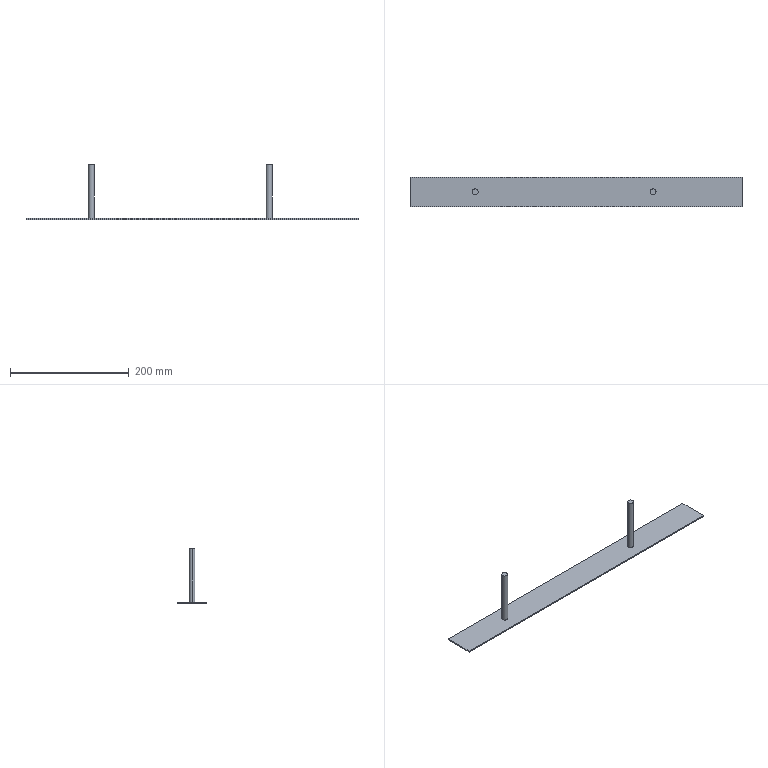Part | STEP file | 1 solid | 12 faces | box 560 x 50 x 93 mm | volume 70294 mm3 | plane 8 | cylinder 4 | commonest cylinder face diameters 10 x4
STEP:
#1=CARTESIAN_POINT('',(0.,0.,0.));
#2=DIRECTION('',(0.,0.,1.));
#3=DIRECTION('',(1.,0.,0.));
#4=AXIS2_PLACEMENT_3D('',#1,#2,#3);
#5=CARTESIAN_POINT('',(125.,0.,2.));
#6=VERTEX_POINT('',#5);
#7=CARTESIAN_POINT('',(135.,0.,2.));
#8=VERTEX_POINT('',#7);
#9=CARTESIAN_POINT('',(130.,0.,2.));
#10=DIRECTION('',(0.,0.,-1.));
#11=DIRECTION('',(1.,0.,0.));
#12=AXIS2_PLACEMENT_3D('',#9,#10,#11);
#13=CIRCLE('',#12,5.);
#14=CARTESIAN_POINT('',(130.,0.,93.));
#15=DIRECTION('',(0.,0.,1.));
#16=DIRECTION('',(1.,0.,0.));
#17=AXIS2_PLACEMENT_3D('',#14,#15,#16);
#18=CYLINDRICAL_SURFACE('',#17,5.);
#19=CARTESIAN_POINT('',(6.283,-91.));
#20=DIRECTION('',(-1.,0.));
#21=VECTOR('',#20,1.);
#22=LINE('',#19,#21);
#23=(GEOMETRIC_REPRESENTATION_CONTEXT(2)PARAMETRIC_REPRESENTATION_CONTEXT()REPRESENTATION_CONTEXT('',''));
#24=DEFINITIONAL_REPRESENTATION('',(#22),#23);
#25=PCURVE('',#18,#24);
#26=CARTESIAN_POINT('',(0.,0.,2.));
#27=DIRECTION('',(0.,0.,1.));
#28=DIRECTION('',(1.,0.,0.));
#29=AXIS2_PLACEMENT_3D('',#26,#27,#28);
#30=PLANE('',#29);
#31=CARTESIAN_POINT('',(135.,0.));
#32=CARTESIAN_POINT('',(135.,-8.66));
#33=CARTESIAN_POINT('',(127.5,-4.33));
#34=CARTESIAN_POINT('',(120.,0.));
#35=CARTESIAN_POINT('',(127.5,4.33));
#36=CARTESIAN_POINT('',(135.,8.66));
#37=CARTESIAN_POINT('',(135.,0.));
#38=(BOUNDED_CURVE()B_SPLINE_CURVE(2,(#31,#32,#33,#34,#35,#36,#37),.UNSPECIFIED.,.T.,.F.)B_SPLINE_CURVE_WITH_KNOTS((1,2,2,2,2,1),(-2.094,0.,2.094,4.189,6.283,8.378),.UNSPECIFIED.)CURVE()GEOMETRIC_REPRESENTATION_ITEM()RATIONAL_B_SPLINE_CURVE((1.,0.5,1.,0.5,1.,0.5,1.))REPRESENTATION_ITEM(''));
#39=(GEOMETRIC_REPRESENTATION_CONTEXT(2)PARAMETRIC_REPRESENTATION_CONTEXT()REPRESENTATION_CONTEXT('',''));
#40=DEFINITIONAL_REPRESENTATION('',(#38),#39);
#41=PCURVE('',#30,#40);
#42=SURFACE_CURVE('',#13,(#25,#41),.PCURVE_S1.);
#43=EDGE_CURVE('',#6,#8,#42,.T.);
#44=ORIENTED_EDGE('',*,*,#43,.F.);
#45=CARTESIAN_POINT('',(125.,0.,93.));
#46=VERTEX_POINT('',#45);
#47=CARTESIAN_POINT('',(125.,0.,93.));
#48=DIRECTION('',(0.,0.,1.));
#49=VECTOR('',#48,1.);
#50=LINE('',#47,#49);
#51=CARTESIAN_POINT('',(3.142,0.));
#52=DIRECTION('',(0.,1.));
#53=VECTOR('',#52,1.);
#54=LINE('',#51,#53);
#55=(GEOMETRIC_REPRESENTATION_CONTEXT(2)PARAMETRIC_REPRESENTATION_CONTEXT()REPRESENTATION_CONTEXT('',''));
#56=DEFINITIONAL_REPRESENTATION('',(#54),#55);
#57=PCURVE('',#18,#56);
#58=CARTESIAN_POINT('',(130.,0.,93.));
#59=DIRECTION('',(0.,0.,1.));
#60=DIRECTION('',(1.,0.,0.));
#61=AXIS2_PLACEMENT_3D('',#58,#59,#60);
#62=CYLINDRICAL_SURFACE('',#61,5.);
#63=CARTESIAN_POINT('',(3.142,0.));
#64=DIRECTION('',(0.,1.));
#65=VECTOR('',#64,1.);
#66=LINE('',#63,#65);
#67=(GEOMETRIC_REPRESENTATION_CONTEXT(2)PARAMETRIC_REPRESENTATION_CONTEXT()REPRESENTATION_CONTEXT('',''));
#68=DEFINITIONAL_REPRESENTATION('',(#66),#67);
#69=PCURVE('',#62,#68);
#70=SURFACE_CURVE('',#50,(#57,#69),.PCURVE_S1.);
#71=EDGE_CURVE('',#6,#46,#70,.T.);
#72=ORIENTED_EDGE('',*,*,#71,.T.);
#73=CARTESIAN_POINT('',(135.,0.,93.));
#74=VERTEX_POINT('',#73);
#75=CARTESIAN_POINT('',(130.,0.,93.));
#76=DIRECTION('',(0.,0.,-1.));
#77=DIRECTION('',(1.,0.,0.));
#78=AXIS2_PLACEMENT_3D('',#75,#76,#77);
#79=CIRCLE('',#78,5.);
#80=CARTESIAN_POINT('',(6.283,0.));
#81=DIRECTION('',(-1.,0.));
#82=VECTOR('',#81,1.);
#83=LINE('',#80,#82);
#84=(GEOMETRIC_REPRESENTATION_CONTEXT(2)PARAMETRIC_REPRESENTATION_CONTEXT()REPRESENTATION_CONTEXT('',''));
#85=DEFINITIONAL_REPRESENTATION('',(#83),#84);
#86=PCURVE('',#18,#85);
#87=CARTESIAN_POINT('',(130.,0.,93.));
#88=DIRECTION('',(0.,0.,1.));
#89=DIRECTION('',(1.,0.,0.));
#90=AXIS2_PLACEMENT_3D('',#87,#88,#89);
#91=PLANE('',#90);
#92=CARTESIAN_POINT('',(5.,0.));
#93=CARTESIAN_POINT('',(5.,-8.66));
#94=CARTESIAN_POINT('',(-2.5,-4.33));
#95=CARTESIAN_POINT('',(-10.,0.));
#96=CARTESIAN_POINT('',(-2.5,4.33));
#97=CARTESIAN_POINT('',(5.,8.66));
#98=CARTESIAN_POINT('',(5.,0.));
#99=(BOUNDED_CURVE()B_SPLINE_CURVE(2,(#92,#93,#94,#95,#96,#97,#98),.UNSPECIFIED.,.T.,.F.)B_SPLINE_CURVE_WITH_KNOTS((1,2,2,2,2,1),(-2.094,0.,2.094,4.189,6.283,8.378),.UNSPECIFIED.)CURVE()GEOMETRIC_REPRESENTATION_ITEM()RATIONAL_B_SPLINE_CURVE((1.,0.5,1.,0.5,1.,0.5,1.))REPRESENTATION_ITEM(''));
#100=(GEOMETRIC_REPRESENTATION_CONTEXT(2)PARAMETRIC_REPRESENTATION_CONTEXT()REPRESENTATION_CONTEXT('',''));
#101=DEFINITIONAL_REPRESENTATION('',(#99),#100);
#102=PCURVE('',#91,#101);
#103=SURFACE_CURVE('',#79,(#86,#102),.PCURVE_S1.);
#104=EDGE_CURVE('',#46,#74,#103,.T.);
#105=ORIENTED_EDGE('',*,*,#104,.T.);
#106=CARTESIAN_POINT('',(135.,0.,93.));
#107=DIRECTION('',(0.,0.,1.));
#108=VECTOR('',#107,1.);
#109=LINE('',#106,#108);
#110=CARTESIAN_POINT('',(0.,0.));
#111=DIRECTION('',(0.,1.));
#112=VECTOR('',#111,1.);
#113=LINE('',#110,#112);
#114=(GEOMETRIC_REPRESENTATION_CONTEXT(2)PARAMETRIC_REPRESENTATION_CONTEXT()REPRESENTATION_CONTEXT('',''));
#115=DEFINITIONAL_REPRESENTATION('',(#113),#114);
#116=PCURVE('',#18,#115);
#117=CARTESIAN_POINT('',(6.283,0.));
#118=DIRECTION('',(0.,1.));
#119=VECTOR('',#118,1.);
#120=LINE('',#117,#119);
#121=(GEOMETRIC_REPRESENTATION_CONTEXT(2)PARAMETRIC_REPRESENTATION_CONTEXT()REPRESENTATION_CONTEXT('',''));
#122=DEFINITIONAL_REPRESENTATION('',(#120),#121);
#123=PCURVE('',#62,#122);
#124=SURFACE_CURVE('',#109,(#116,#123),.PCURVE_S1.);
#125=EDGE_CURVE('',#8,#74,#124,.T.);
#126=ORIENTED_EDGE('',*,*,#125,.F.);
#127=EDGE_LOOP('',(#44,#72,#105,#126));
#128=FACE_BOUND('',#127,.T.);
#129=ADVANCED_FACE('',(#128),#18,.T.);
#130=CARTESIAN_POINT('',(-175.,0.,2.));
#131=VERTEX_POINT('',#130);
#132=CARTESIAN_POINT('',(-165.,0.,2.));
#133=VERTEX_POINT('',#132);
#134=CARTESIAN_POINT('',(-170.,0.,2.));
#135=DIRECTION('',(0.,0.,-1.));
#136=DIRECTION('',(1.,0.,0.));
#137=AXIS2_PLACEMENT_3D('',#134,#135,#136);
#138=CIRCLE('',#137,5.);
#139=CARTESIAN_POINT('',(-170.,0.,93.));
#140=DIRECTION('',(0.,0.,1.));
#141=DIRECTION('',(1.,0.,0.));
#142=AXIS2_PLACEMENT_3D('',#139,#140,#141);
#143=CYLINDRICAL_SURFACE('',#142,5.);
#144=CARTESIAN_POINT('',(6.283,-91.));
#145=DIRECTION('',(-1.,0.));
#146=VECTOR('',#145,1.);
#147=LINE('',#144,#146);
#148=(GEOMETRIC_REPRESENTATION_CONTEXT(2)PARAMETRIC_REPRESENTATION_CONTEXT()REPRESENTATION_CONTEXT('',''));
#149=DEFINITIONAL_REPRESENTATION('',(#147),#148);
#150=PCURVE('',#143,#149);
#151=CARTESIAN_POINT('',(-165.,0.));
#152=CARTESIAN_POINT('',(-165.,-8.66));
#153=CARTESIAN_POINT('',(-172.5,-4.33));
#154=CARTESIAN_POINT('',(-180.,0.));
#155=CARTESIAN_POINT('',(-172.5,4.33));
#156=CARTESIAN_POINT('',(-165.,8.66));
#157=CARTESIAN_POINT('',(-165.,0.));
#158=(BOUNDED_CURVE()B_SPLINE_CURVE(2,(#151,#152,#153,#154,#155,#156,#157),.UNSPECIFIED.,.T.,.F.)B_SPLINE_CURVE_WITH_KNOTS((1,2,2,2,2,1),(-2.094,0.,2.094,4.189,6.283,8.378),.UNSPECIFIED.)CURVE()GEOMETRIC_REPRESENTATION_ITEM()RATIONAL_B_SPLINE_CURVE((1.,0.5,1.,0.5,1.,0.5,1.))REPRESENTATION_ITEM(''));
#159=(GEOMETRIC_REPRESENTATION_CONTEXT(2)PARAMETRIC_REPRESENTATION_CONTEXT()REPRESENTATION_CONTEXT('',''));
#160=DEFINITIONAL_REPRESENTATION('',(#158),#159);
#161=PCURVE('',#30,#160);
#162=SURFACE_CURVE('',#138,(#150,#161),.PCURVE_S1.);
#163=EDGE_CURVE('',#131,#133,#162,.T.);
#164=ORIENTED_EDGE('',*,*,#163,.F.);
#165=CARTESIAN_POINT('',(-175.,0.,93.));
#166=VERTEX_POINT('',#165);
#167=CARTESIAN_POINT('',(-175.,0.,93.));
#168=DIRECTION('',(0.,0.,1.));
#169=VECTOR('',#168,1.);
#170=LINE('',#167,#169);
#171=CARTESIAN_POINT('',(3.142,0.));
#172=DIRECTION('',(0.,1.));
#173=VECTOR('',#172,1.);
#174=LINE('',#171,#173);
#175=(GEOMETRIC_REPRESENTATION_CONTEXT(2)PARAMETRIC_REPRESENTATION_CONTEXT()REPRESENTATION_CONTEXT('',''));
#176=DEFINITIONAL_REPRESENTATION('',(#174),#175);
#177=PCURVE('',#143,#176);
#178=CARTESIAN_POINT('',(-170.,0.,93.));
#179=DIRECTION('',(0.,0.,1.));
#180=DIRECTION('',(1.,0.,0.));
#181=AXIS2_PLACEMENT_3D('',#178,#179,#180);
#182=CYLINDRICAL_SURFACE('',#181,5.);
#183=CARTESIAN_POINT('',(3.142,0.));
#184=DIRECTION('',(0.,1.));
#185=VECTOR('',#184,1.);
#186=LINE('',#183,#185);
#187=(GEOMETRIC_REPRESENTATION_CONTEXT(2)PARAMETRIC_REPRESENTATION_CONTEXT()REPRESENTATION_CONTEXT('',''));
#188=DEFINITIONAL_REPRESENTATION('',(#186),#187);
#189=PCURVE('',#182,#188);
#190=SURFACE_CURVE('',#170,(#177,#189),.PCURVE_S1.);
#191=EDGE_CURVE('',#131,#166,#190,.T.);
#192=ORIENTED_EDGE('',*,*,#191,.T.);
#193=CARTESIAN_POINT('',(-165.,0.,93.));
#194=VERTEX_POINT('',#193);
#195=CARTESIAN_POINT('',(-170.,0.,93.));
#196=DIRECTION('',(0.,0.,-1.));
#197=DIRECTION('',(1.,0.,0.));
#198=AXIS2_PLACEMENT_3D('',#195,#196,#197);
#199=CIRCLE('',#198,5.);
#200=CARTESIAN_POINT('',(6.283,0.));
#201=DIRECTION('',(-1.,0.));
#202=VECTOR('',#201,1.);
#203=LINE('',#200,#202);
#204=(GEOMETRIC_REPRESENTATION_CONTEXT(2)PARAMETRIC_REPRESENTATION_CONTEXT()REPRESENTATION_CONTEXT('',''));
#205=DEFINITIONAL_REPRESENTATION('',(#203),#204);
#206=PCURVE('',#143,#205);
#207=CARTESIAN_POINT('',(-170.,0.,93.));
#208=DIRECTION('',(0.,0.,1.));
#209=DIRECTION('',(1.,0.,0.));
#210=AXIS2_PLACEMENT_3D('',#207,#208,#209);
#211=PLANE('',#210);
#212=CARTESIAN_POINT('',(5.,0.));
#213=CARTESIAN_POINT('',(5.,-8.66));
#214=CARTESIAN_POINT('',(-2.5,-4.33));
#215=CARTESIAN_POINT('',(-10.,0.));
#216=CARTESIAN_POINT('',(-2.5,4.33));
#217=CARTESIAN_POINT('',(5.,8.66));
#218=CARTESIAN_POINT('',(5.,0.));
#219=(BOUNDED_CURVE()B_SPLINE_CURVE(2,(#212,#213,#214,#215,#216,#217,#218),.UNSPECIFIED.,.T.,.F.)B_SPLINE_CURVE_WITH_KNOTS((1,2,2,2,2,1),(-2.094,0.,2.094,4.189,6.283,8.378),.UNSPECIFIED.)CURVE()GEOMETRIC_REPRESENTATION_ITEM()RATIONAL_B_SPLINE_CURVE((1.,0.5,1.,0.5,1.,0.5,1.))REPRESENTATION_ITEM(''));
#220=(GEOMETRIC_REPRESENTATION_CONTEXT(2)PARAMETRIC_REPRESENTATION_CONTEXT()REPRESENTATION_CONTEXT('',''));
#221=DEFINITIONAL_REPRESENTATION('',(#219),#220);
#222=PCURVE('',#211,#221);
#223=SURFACE_CURVE('',#199,(#206,#222),.PCURVE_S1.);
#224=EDGE_CURVE('',#166,#194,#223,.T.);
#225=ORIENTED_EDGE('',*,*,#224,.T.);
#226=CARTESIAN_POINT('',(-165.,0.,93.));
#227=DIRECTION('',(0.,0.,1.));
#228=VECTOR('',#227,1.);
#229=LINE('',#226,#228);
#230=CARTESIAN_POINT('',(0.,0.));
#231=DIRECTION('',(0.,1.));
#232=VECTOR('',#231,1.);
#233=LINE('',#230,#232);
#234=(GEOMETRIC_REPRESENTATION_CONTEXT(2)PARAMETRIC_REPRESENTATION_CONTEXT()REPRESENTATION_CONTEXT('',''));
#235=DEFINITIONAL_REPRESENTATION('',(#233),#234);
#236=PCURVE('',#143,#235);
#237=CARTESIAN_POINT('',(6.283,0.));
#238=DIRECTION('',(0.,1.));
#239=VECTOR('',#238,1.);
#240=LINE('',#237,#239);
#241=(GEOMETRIC_REPRESENTATION_CONTEXT(2)PARAMETRIC_REPRESENTATION_CONTEXT()REPRESENTATION_CONTEXT('',''));
#242=DEFINITIONAL_REPRESENTATION('',(#240),#241);
#243=PCURVE('',#182,#242);
#244=SURFACE_CURVE('',#229,(#236,#243),.PCURVE_S1.);
#245=EDGE_CURVE('',#133,#194,#244,.T.);
#246=ORIENTED_EDGE('',*,*,#245,.F.);
#247=EDGE_LOOP('',(#164,#192,#225,#246));
#248=FACE_BOUND('',#247,.T.);
#249=ADVANCED_FACE('',(#248),#143,.T.);
#250=CARTESIAN_POINT('',(-280.,-25.,0.));
#251=VERTEX_POINT('',#250);
#252=CARTESIAN_POINT('',(280.,-25.,0.));
#253=VERTEX_POINT('',#252);
#254=CARTESIAN_POINT('',(0.,-25.,0.));
#255=DIRECTION('',(1.,0.,0.));
#256=VECTOR('',#255,1.);
#257=LINE('',#254,#256);
#258=CARTESIAN_POINT('',(0.,0.,0.));
#259=DIRECTION('',(0.,0.,1.));
#260=DIRECTION('',(1.,0.,0.));
#261=AXIS2_PLACEMENT_3D('',#258,#259,#260);
#262=PLANE('',#261);
#263=CARTESIAN_POINT('',(0.,-25.));
#264=DIRECTION('',(1.,0.));
#265=VECTOR('',#264,1.);
#266=LINE('',#263,#265);
#267=(GEOMETRIC_REPRESENTATION_CONTEXT(2)PARAMETRIC_REPRESENTATION_CONTEXT()REPRESENTATION_CONTEXT('',''));
#268=DEFINITIONAL_REPRESENTATION('',(#266),#267);
#269=PCURVE('',#262,#268);
#270=CARTESIAN_POINT('',(-280.,-25.,2.));
#271=DIRECTION('',(0.,1.,0.));
#272=DIRECTION('',(0.,0.,1.));
#273=AXIS2_PLACEMENT_3D('',#270,#271,#272);
#274=PLANE('',#273);
#275=CARTESIAN_POINT('',(-2.,280.));
#276=DIRECTION('',(0.,1.));
#277=VECTOR('',#276,1.);
#278=LINE('',#275,#277);
#279=(GEOMETRIC_REPRESENTATION_CONTEXT(2)PARAMETRIC_REPRESENTATION_CONTEXT()REPRESENTATION_CONTEXT('',''));
#280=DEFINITIONAL_REPRESENTATION('',(#278),#279);
#281=PCURVE('',#274,#280);
#282=SURFACE_CURVE('',#257,(#269,#281),.PCURVE_S1.);
#283=EDGE_CURVE('',#251,#253,#282,.T.);
#284=ORIENTED_EDGE('',*,*,#283,.F.);
#285=CARTESIAN_POINT('',(-280.,25.,0.));
#286=VERTEX_POINT('',#285);
#287=CARTESIAN_POINT('',(-280.,0.,0.));
#288=DIRECTION('',(0.,-1.,0.));
#289=VECTOR('',#288,1.);
#290=LINE('',#287,#289);
#291=CARTESIAN_POINT('',(-280.,0.));
#292=DIRECTION('',(0.,-1.));
#293=VECTOR('',#292,1.);
#294=LINE('',#291,#293);
#295=(GEOMETRIC_REPRESENTATION_CONTEXT(2)PARAMETRIC_REPRESENTATION_CONTEXT()REPRESENTATION_CONTEXT('',''));
#296=DEFINITIONAL_REPRESENTATION('',(#294),#295);
#297=PCURVE('',#262,#296);
#298=CARTESIAN_POINT('',(-280.,25.,2.));
#299=DIRECTION('',(1.,0.,0.));
#300=DIRECTION('',(0.,0.,-1.));
#301=AXIS2_PLACEMENT_3D('',#298,#299,#300);
#302=PLANE('',#301);
#303=CARTESIAN_POINT('',(2.,-25.));
#304=DIRECTION('',(0.,-1.));
#305=VECTOR('',#304,1.);
#306=LINE('',#303,#305);
#307=(GEOMETRIC_REPRESENTATION_CONTEXT(2)PARAMETRIC_REPRESENTATION_CONTEXT()REPRESENTATION_CONTEXT('',''));
#308=DEFINITIONAL_REPRESENTATION('',(#306),#307);
#309=PCURVE('',#302,#308);
#310=SURFACE_CURVE('',#290,(#297,#309),.PCURVE_S1.);
#311=EDGE_CURVE('',#286,#251,#310,.T.);
#312=ORIENTED_EDGE('',*,*,#311,.F.);
#313=CARTESIAN_POINT('',(280.,25.,0.));
#314=VERTEX_POINT('',#313);
#315=CARTESIAN_POINT('',(0.,25.,0.));
#316=DIRECTION('',(-1.,0.,0.));
#317=VECTOR('',#316,1.);
#318=LINE('',#315,#317);
#319=CARTESIAN_POINT('',(0.,25.));
#320=DIRECTION('',(-1.,0.));
#321=VECTOR('',#320,1.);
#322=LINE('',#319,#321);
#323=(GEOMETRIC_REPRESENTATION_CONTEXT(2)PARAMETRIC_REPRESENTATION_CONTEXT()REPRESENTATION_CONTEXT('',''));
#324=DEFINITIONAL_REPRESENTATION('',(#322),#323);
#325=PCURVE('',#262,#324);
#326=CARTESIAN_POINT('',(-280.,25.,2.));
#327=DIRECTION('',(0.,-1.,0.));
#328=DIRECTION('',(0.,0.,-1.));
#329=AXIS2_PLACEMENT_3D('',#326,#327,#328);
#330=PLANE('',#329);
#331=CARTESIAN_POINT('',(2.,280.));
#332=DIRECTION('',(0.,-1.));
#333=VECTOR('',#332,1.);
#334=LINE('',#331,#333);
#335=(GEOMETRIC_REPRESENTATION_CONTEXT(2)PARAMETRIC_REPRESENTATION_CONTEXT()REPRESENTATION_CONTEXT('',''));
#336=DEFINITIONAL_REPRESENTATION('',(#334),#335);
#337=PCURVE('',#330,#336);
#338=SURFACE_CURVE('',#318,(#325,#337),.PCURVE_S1.);
#339=EDGE_CURVE('',#314,#286,#338,.T.);
#340=ORIENTED_EDGE('',*,*,#339,.F.);
#341=CARTESIAN_POINT('',(280.,0.,0.));
#342=DIRECTION('',(0.,1.,0.));
#343=VECTOR('',#342,1.);
#344=LINE('',#341,#343);
#345=CARTESIAN_POINT('',(280.,0.));
#346=DIRECTION('',(0.,1.));
#347=VECTOR('',#346,1.);
#348=LINE('',#345,#347);
#349=(GEOMETRIC_REPRESENTATION_CONTEXT(2)PARAMETRIC_REPRESENTATION_CONTEXT()REPRESENTATION_CONTEXT('',''));
#350=DEFINITIONAL_REPRESENTATION('',(#348),#349);
#351=PCURVE('',#262,#350);
#352=CARTESIAN_POINT('',(280.,25.,2.));
#353=DIRECTION('',(-1.,0.,0.));
#354=DIRECTION('',(0.,0.,1.));
#355=AXIS2_PLACEMENT_3D('',#352,#353,#354);
#356=PLANE('',#355);
#357=CARTESIAN_POINT('',(-2.,-25.));
#358=DIRECTION('',(0.,1.));
#359=VECTOR('',#358,1.);
#360=LINE('',#357,#359);
#361=(GEOMETRIC_REPRESENTATION_CONTEXT(2)PARAMETRIC_REPRESENTATION_CONTEXT()REPRESENTATION_CONTEXT('',''));
#362=DEFINITIONAL_REPRESENTATION('',(#360),#361);
#363=PCURVE('',#356,#362);
#364=SURFACE_CURVE('',#344,(#351,#363),.PCURVE_S1.);
#365=EDGE_CURVE('',#253,#314,#364,.T.);
#366=ORIENTED_EDGE('',*,*,#365,.F.);
#367=EDGE_LOOP('',(#284,#312,#340,#366));
#368=FACE_BOUND('',#367,.T.);
#369=ADVANCED_FACE('',(#368),#262,.F.);
#370=CARTESIAN_POINT('',(280.,25.,2.));
#371=VERTEX_POINT('',#370);
#372=CARTESIAN_POINT('',(280.,25.,2.));
#373=DIRECTION('',(0.,0.,-1.));
#374=VECTOR('',#373,1.);
#375=LINE('',#372,#374);
#376=CARTESIAN_POINT('',(0.,0.));
#377=DIRECTION('',(-1.,0.));
#378=VECTOR('',#377,1.);
#379=LINE('',#376,#378);
#380=(GEOMETRIC_REPRESENTATION_CONTEXT(2)PARAMETRIC_REPRESENTATION_CONTEXT()REPRESENTATION_CONTEXT('',''));
#381=DEFINITIONAL_REPRESENTATION('',(#379),#380);
#382=PCURVE('',#356,#381);
#383=CARTESIAN_POINT('',(0.,560.));
#384=DIRECTION('',(1.,0.));
#385=VECTOR('',#384,1.);
#386=LINE('',#383,#385);
#387=(GEOMETRIC_REPRESENTATION_CONTEXT(2)PARAMETRIC_REPRESENTATION_CONTEXT()REPRESENTATION_CONTEXT('',''));
#388=DEFINITIONAL_REPRESENTATION('',(#386),#387);
#389=PCURVE('',#330,#388);
#390=SURFACE_CURVE('',#375,(#382,#389),.PCURVE_S1.);
#391=EDGE_CURVE('',#371,#314,#390,.T.);
#392=ORIENTED_EDGE('',*,*,#391,.F.);
#393=CARTESIAN_POINT('',(280.,-25.,2.));
#394=VERTEX_POINT('',#393);
#395=CARTESIAN_POINT('',(280.,25.,2.));
#396=DIRECTION('',(0.,1.,0.));
#397=VECTOR('',#396,1.);
#398=LINE('',#395,#397);
#399=CARTESIAN_POINT('',(0.,0.));
#400=DIRECTION('',(0.,1.));
#401=VECTOR('',#400,1.);
#402=LINE('',#399,#401);
#403=(GEOMETRIC_REPRESENTATION_CONTEXT(2)PARAMETRIC_REPRESENTATION_CONTEXT()REPRESENTATION_CONTEXT('',''));
#404=DEFINITIONAL_REPRESENTATION('',(#402),#403);
#405=PCURVE('',#356,#404);
#406=CARTESIAN_POINT('',(280.,25.));
#407=DIRECTION('',(0.,1.));
#408=VECTOR('',#407,1.);
#409=LINE('',#406,#408);
#410=(GEOMETRIC_REPRESENTATION_CONTEXT(2)PARAMETRIC_REPRESENTATION_CONTEXT()REPRESENTATION_CONTEXT('',''));
#411=DEFINITIONAL_REPRESENTATION('',(#409),#410);
#412=PCURVE('',#30,#411);
#413=SURFACE_CURVE('',#398,(#405,#412),.PCURVE_S1.);
#414=EDGE_CURVE('',#394,#371,#413,.T.);
#415=ORIENTED_EDGE('',*,*,#414,.F.);
#416=CARTESIAN_POINT('',(280.,-25.,2.));
#417=DIRECTION('',(0.,0.,1.));
#418=VECTOR('',#417,1.);
#419=LINE('',#416,#418);
#420=CARTESIAN_POINT('',(0.,-50.));
#421=DIRECTION('',(1.,0.));
#422=VECTOR('',#421,1.);
#423=LINE('',#420,#422);
#424=(GEOMETRIC_REPRESENTATION_CONTEXT(2)PARAMETRIC_REPRESENTATION_CONTEXT()REPRESENTATION_CONTEXT('',''));
#425=DEFINITIONAL_REPRESENTATION('',(#423),#424);
#426=PCURVE('',#356,#425);
#427=CARTESIAN_POINT('',(0.,560.));
#428=DIRECTION('',(1.,0.));
#429=VECTOR('',#428,1.);
#430=LINE('',#427,#429);
#431=(GEOMETRIC_REPRESENTATION_CONTEXT(2)PARAMETRIC_REPRESENTATION_CONTEXT()REPRESENTATION_CONTEXT('',''));
#432=DEFINITIONAL_REPRESENTATION('',(#430),#431);
#433=PCURVE('',#274,#432);
#434=SURFACE_CURVE('',#419,(#426,#433),.PCURVE_S1.);
#435=EDGE_CURVE('',#253,#394,#434,.T.);
#436=ORIENTED_EDGE('',*,*,#435,.F.);
#437=ORIENTED_EDGE('',*,*,#365,.T.);
#438=EDGE_LOOP('',(#392,#415,#436,#437));
#439=FACE_BOUND('',#438,.T.);
#440=ADVANCED_FACE('',(#439),#356,.F.);
#441=ORIENTED_EDGE('',*,*,#435,.T.);
#442=CARTESIAN_POINT('',(-280.,-25.,2.));
#443=VERTEX_POINT('',#442);
#444=CARTESIAN_POINT('',(-280.,-25.,2.));
#445=DIRECTION('',(1.,0.,0.));
#446=VECTOR('',#445,1.);
#447=LINE('',#444,#446);
#448=CARTESIAN_POINT('',(0.,0.));
#449=DIRECTION('',(0.,1.));
#450=VECTOR('',#449,1.);
#451=LINE('',#448,#450);
#452=(GEOMETRIC_REPRESENTATION_CONTEXT(2)PARAMETRIC_REPRESENTATION_CONTEXT()REPRESENTATION_CONTEXT('',''));
#453=DEFINITIONAL_REPRESENTATION('',(#451),#452);
#454=PCURVE('',#274,#453);
#455=CARTESIAN_POINT('',(-280.,-25.));
#456=DIRECTION('',(1.,0.));
#457=VECTOR('',#456,1.);
#458=LINE('',#455,#457);
#459=(GEOMETRIC_REPRESENTATION_CONTEXT(2)PARAMETRIC_REPRESENTATION_CONTEXT()REPRESENTATION_CONTEXT('',''));
#460=DEFINITIONAL_REPRESENTATION('',(#458),#459);
#461=PCURVE('',#30,#460);
#462=SURFACE_CURVE('',#447,(#454,#461),.PCURVE_S1.);
#463=EDGE_CURVE('',#443,#394,#462,.T.);
#464=ORIENTED_EDGE('',*,*,#463,.F.);
#465=CARTESIAN_POINT('',(-280.,-25.,2.));
#466=DIRECTION('',(0.,0.,1.));
#467=VECTOR('',#466,1.);
#468=LINE('',#465,#467);
#469=CARTESIAN_POINT('',(0.,0.));
#470=DIRECTION('',(1.,0.));
#471=VECTOR('',#470,1.);
#472=LINE('',#469,#471);
#473=(GEOMETRIC_REPRESENTATION_CONTEXT(2)PARAMETRIC_REPRESENTATION_CONTEXT()REPRESENTATION_CONTEXT('',''));
#474=DEFINITIONAL_REPRESENTATION('',(#472),#473);
#475=PCURVE('',#274,#474);
#476=CARTESIAN_POINT('',(0.,-50.));
#477=DIRECTION('',(-1.,0.));
#478=VECTOR('',#477,1.);
#479=LINE('',#476,#478);
#480=(GEOMETRIC_REPRESENTATION_CONTEXT(2)PARAMETRIC_REPRESENTATION_CONTEXT()REPRESENTATION_CONTEXT('',''));
#481=DEFINITIONAL_REPRESENTATION('',(#479),#480);
#482=PCURVE('',#302,#481);
#483=SURFACE_CURVE('',#468,(#475,#482),.PCURVE_S1.);
#484=EDGE_CURVE('',#251,#443,#483,.T.);
#485=ORIENTED_EDGE('',*,*,#484,.F.);
#486=ORIENTED_EDGE('',*,*,#283,.T.);
#487=EDGE_LOOP('',(#441,#464,#485,#486));
#488=FACE_BOUND('',#487,.T.);
#489=ADVANCED_FACE('',(#488),#274,.F.);
#490=ORIENTED_EDGE('',*,*,#484,.T.);
#491=CARTESIAN_POINT('',(-280.,25.,2.));
#492=VERTEX_POINT('',#491);
#493=CARTESIAN_POINT('',(-280.,25.,2.));
#494=DIRECTION('',(0.,-1.,0.));
#495=VECTOR('',#494,1.);
#496=LINE('',#493,#495);
#497=CARTESIAN_POINT('',(0.,0.));
#498=DIRECTION('',(0.,-1.));
#499=VECTOR('',#498,1.);
#500=LINE('',#497,#499);
#501=(GEOMETRIC_REPRESENTATION_CONTEXT(2)PARAMETRIC_REPRESENTATION_CONTEXT()REPRESENTATION_CONTEXT('',''));
#502=DEFINITIONAL_REPRESENTATION('',(#500),#501);
#503=PCURVE('',#302,#502);
#504=CARTESIAN_POINT('',(-280.,25.));
#505=DIRECTION('',(0.,-1.));
#506=VECTOR('',#505,1.);
#507=LINE('',#504,#506);
#508=(GEOMETRIC_REPRESENTATION_CONTEXT(2)PARAMETRIC_REPRESENTATION_CONTEXT()REPRESENTATION_CONTEXT('',''));
#509=DEFINITIONAL_REPRESENTATION('',(#507),#508);
#510=PCURVE('',#30,#509);
#511=SURFACE_CURVE('',#496,(#503,#510),.PCURVE_S1.);
#512=EDGE_CURVE('',#492,#443,#511,.T.);
#513=ORIENTED_EDGE('',*,*,#512,.F.);
#514=CARTESIAN_POINT('',(-280.,25.,2.));
#515=DIRECTION('',(0.,0.,1.));
#516=VECTOR('',#515,1.);
#517=LINE('',#514,#516);
#518=CARTESIAN_POINT('',(0.,0.));
#519=DIRECTION('',(-1.,0.));
#520=VECTOR('',#519,1.);
#521=LINE('',#518,#520);
#522=(GEOMETRIC_REPRESENTATION_CONTEXT(2)PARAMETRIC_REPRESENTATION_CONTEXT()REPRESENTATION_CONTEXT('',''));
#523=DEFINITIONAL_REPRESENTATION('',(#521),#522);
#524=PCURVE('',#302,#523);
#525=CARTESIAN_POINT('',(0.,0.));
#526=DIRECTION('',(-1.,0.));
#527=VECTOR('',#526,1.);
#528=LINE('',#525,#527);
#529=(GEOMETRIC_REPRESENTATION_CONTEXT(2)PARAMETRIC_REPRESENTATION_CONTEXT()REPRESENTATION_CONTEXT('',''));
#530=DEFINITIONAL_REPRESENTATION('',(#528),#529);
#531=PCURVE('',#330,#530);
#532=SURFACE_CURVE('',#517,(#524,#531),.PCURVE_S1.);
#533=EDGE_CURVE('',#286,#492,#532,.T.);
#534=ORIENTED_EDGE('',*,*,#533,.F.);
#535=ORIENTED_EDGE('',*,*,#311,.T.);
#536=EDGE_LOOP('',(#490,#513,#534,#535));
#537=FACE_BOUND('',#536,.T.);
#538=ADVANCED_FACE('',(#537),#302,.F.);
#539=ORIENTED_EDGE('',*,*,#533,.T.);
#540=CARTESIAN_POINT('',(-280.,25.,2.));
#541=DIRECTION('',(-1.,0.,0.));
#542=VECTOR('',#541,1.);
#543=LINE('',#540,#542);
#544=CARTESIAN_POINT('',(0.,0.));
#545=DIRECTION('',(0.,-1.));
#546=VECTOR('',#545,1.);
#547=LINE('',#544,#546);
#548=(GEOMETRIC_REPRESENTATION_CONTEXT(2)PARAMETRIC_REPRESENTATION_CONTEXT()REPRESENTATION_CONTEXT('',''));
#549=DEFINITIONAL_REPRESENTATION('',(#547),#548);
#550=PCURVE('',#330,#549);
#551=CARTESIAN_POINT('',(-280.,25.));
#552=DIRECTION('',(-1.,0.));
#553=VECTOR('',#552,1.);
#554=LINE('',#551,#553);
#555=(GEOMETRIC_REPRESENTATION_CONTEXT(2)PARAMETRIC_REPRESENTATION_CONTEXT()REPRESENTATION_CONTEXT('',''));
#556=DEFINITIONAL_REPRESENTATION('',(#554),#555);
#557=PCURVE('',#30,#556);
#558=SURFACE_CURVE('',#543,(#550,#557),.PCURVE_S1.);
#559=EDGE_CURVE('',#371,#492,#558,.T.);
#560=ORIENTED_EDGE('',*,*,#559,.F.);
#561=ORIENTED_EDGE('',*,*,#391,.T.);
#562=ORIENTED_EDGE('',*,*,#339,.T.);
#563=EDGE_LOOP('',(#539,#560,#561,#562));
#564=FACE_BOUND('',#563,.T.);
#565=ADVANCED_FACE('',(#564),#330,.F.);
#566=CARTESIAN_POINT('',(130.,0.,2.));
#567=DIRECTION('',(0.,0.,-1.));
#568=DIRECTION('',(1.,0.,0.));
#569=AXIS2_PLACEMENT_3D('',#566,#567,#568);
#570=CIRCLE('',#569,5.);
#571=CARTESIAN_POINT('',(135.,0.));
#572=CARTESIAN_POINT('',(135.,-8.66));
#573=CARTESIAN_POINT('',(127.5,-4.33));
#574=CARTESIAN_POINT('',(120.,0.));
#575=CARTESIAN_POINT('',(127.5,4.33));
#576=CARTESIAN_POINT('',(135.,8.66));
#577=CARTESIAN_POINT('',(135.,0.));
#578=(BOUNDED_CURVE()B_SPLINE_CURVE(2,(#571,#572,#573,#574,#575,#576,#577),.UNSPECIFIED.,.T.,.F.)B_SPLINE_CURVE_WITH_KNOTS((1,2,2,2,2,1),(-2.094,0.,2.094,4.189,6.283,8.378),.UNSPECIFIED.)CURVE()GEOMETRIC_REPRESENTATION_ITEM()RATIONAL_B_SPLINE_CURVE((1.,0.5,1.,0.5,1.,0.5,1.))REPRESENTATION_ITEM(''));
#579=(GEOMETRIC_REPRESENTATION_CONTEXT(2)PARAMETRIC_REPRESENTATION_CONTEXT()REPRESENTATION_CONTEXT('',''));
#580=DEFINITIONAL_REPRESENTATION('',(#578),#579);
#581=PCURVE('',#30,#580);
#582=CARTESIAN_POINT('',(6.283,-91.));
#583=DIRECTION('',(-1.,0.));
#584=VECTOR('',#583,1.);
#585=LINE('',#582,#584);
#586=(GEOMETRIC_REPRESENTATION_CONTEXT(2)PARAMETRIC_REPRESENTATION_CONTEXT()REPRESENTATION_CONTEXT('',''));
#587=DEFINITIONAL_REPRESENTATION('',(#585),#586);
#588=PCURVE('',#62,#587);
#589=SURFACE_CURVE('',#570,(#581,#588),.PCURVE_S1.);
#590=EDGE_CURVE('',#8,#6,#589,.T.);
#591=ORIENTED_EDGE('',*,*,#590,.T.);
#592=ORIENTED_EDGE('',*,*,#43,.T.);
#593=EDGE_LOOP('',(#591,#592));
#594=FACE_BOUND('',#593,.T.);
#595=CARTESIAN_POINT('',(-170.,0.,2.));
#596=DIRECTION('',(0.,0.,-1.));
#597=DIRECTION('',(1.,0.,0.));
#598=AXIS2_PLACEMENT_3D('',#595,#596,#597);
#599=CIRCLE('',#598,5.);
#600=CARTESIAN_POINT('',(-165.,0.));
#601=CARTESIAN_POINT('',(-165.,-8.66));
#602=CARTESIAN_POINT('',(-172.5,-4.33));
#603=CARTESIAN_POINT('',(-180.,0.));
#604=CARTESIAN_POINT('',(-172.5,4.33));
#605=CARTESIAN_POINT('',(-165.,8.66));
#606=CARTESIAN_POINT('',(-165.,0.));
#607=(BOUNDED_CURVE()B_SPLINE_CURVE(2,(#600,#601,#602,#603,#604,#605,#606),.UNSPECIFIED.,.T.,.F.)B_SPLINE_CURVE_WITH_KNOTS((1,2,2,2,2,1),(-2.094,0.,2.094,4.189,6.283,8.378),.UNSPECIFIED.)CURVE()GEOMETRIC_REPRESENTATION_ITEM()RATIONAL_B_SPLINE_CURVE((1.,0.5,1.,0.5,1.,0.5,1.))REPRESENTATION_ITEM(''));
#608=(GEOMETRIC_REPRESENTATION_CONTEXT(2)PARAMETRIC_REPRESENTATION_CONTEXT()REPRESENTATION_CONTEXT('',''));
#609=DEFINITIONAL_REPRESENTATION('',(#607),#608);
#610=PCURVE('',#30,#609);
#611=CARTESIAN_POINT('',(6.283,-91.));
#612=DIRECTION('',(-1.,0.));
#613=VECTOR('',#612,1.);
#614=LINE('',#611,#613);
#615=(GEOMETRIC_REPRESENTATION_CONTEXT(2)PARAMETRIC_REPRESENTATION_CONTEXT()REPRESENTATION_CONTEXT('',''));
#616=DEFINITIONAL_REPRESENTATION('',(#614),#615);
#617=PCURVE('',#182,#616);
#618=SURFACE_CURVE('',#599,(#610,#617),.PCURVE_S1.);
#619=EDGE_CURVE('',#133,#131,#618,.T.);
#620=ORIENTED_EDGE('',*,*,#619,.T.);
#621=ORIENTED_EDGE('',*,*,#163,.T.);
#622=EDGE_LOOP('',(#620,#621));
#623=FACE_BOUND('',#622,.T.);
#624=ORIENTED_EDGE('',*,*,#512,.T.);
#625=ORIENTED_EDGE('',*,*,#463,.T.);
#626=ORIENTED_EDGE('',*,*,#414,.T.);
#627=ORIENTED_EDGE('',*,*,#559,.T.);
#628=EDGE_LOOP('',(#624,#625,#626,#627));
#629=FACE_BOUND('',#628,.T.);
#630=ADVANCED_FACE('',(#594,#623,#629),#30,.T.);
#631=ORIENTED_EDGE('',*,*,#71,.F.);
#632=ORIENTED_EDGE('',*,*,#590,.F.);
#633=ORIENTED_EDGE('',*,*,#125,.T.);
#634=CARTESIAN_POINT('',(130.,0.,93.));
#635=DIRECTION('',(0.,0.,-1.));
#636=DIRECTION('',(1.,0.,0.));
#637=AXIS2_PLACEMENT_3D('',#634,#635,#636);
#638=CIRCLE('',#637,5.);
#639=CARTESIAN_POINT('',(6.283,0.));
#640=DIRECTION('',(-1.,0.));
#641=VECTOR('',#640,1.);
#642=LINE('',#639,#641);
#643=(GEOMETRIC_REPRESENTATION_CONTEXT(2)PARAMETRIC_REPRESENTATION_CONTEXT()REPRESENTATION_CONTEXT('',''));
#644=DEFINITIONAL_REPRESENTATION('',(#642),#643);
#645=PCURVE('',#62,#644);
#646=CARTESIAN_POINT('',(5.,0.));
#647=CARTESIAN_POINT('',(5.,-8.66));
#648=CARTESIAN_POINT('',(-2.5,-4.33));
#649=CARTESIAN_POINT('',(-10.,0.));
#650=CARTESIAN_POINT('',(-2.5,4.33));
#651=CARTESIAN_POINT('',(5.,8.66));
#652=CARTESIAN_POINT('',(5.,0.));
#653=(BOUNDED_CURVE()B_SPLINE_CURVE(2,(#646,#647,#648,#649,#650,#651,#652),.UNSPECIFIED.,.T.,.F.)B_SPLINE_CURVE_WITH_KNOTS((1,2,2,2,2,1),(-2.094,0.,2.094,4.189,6.283,8.378),.UNSPECIFIED.)CURVE()GEOMETRIC_REPRESENTATION_ITEM()RATIONAL_B_SPLINE_CURVE((1.,0.5,1.,0.5,1.,0.5,1.))REPRESENTATION_ITEM(''));
#654=(GEOMETRIC_REPRESENTATION_CONTEXT(2)PARAMETRIC_REPRESENTATION_CONTEXT()REPRESENTATION_CONTEXT('',''));
#655=DEFINITIONAL_REPRESENTATION('',(#653),#654);
#656=PCURVE('',#91,#655);
#657=SURFACE_CURVE('',#638,(#645,#656),.PCURVE_S1.);
#658=EDGE_CURVE('',#74,#46,#657,.T.);
#659=ORIENTED_EDGE('',*,*,#658,.T.);
#660=EDGE_LOOP('',(#631,#632,#633,#659));
#661=FACE_BOUND('',#660,.T.);
#662=ADVANCED_FACE('',(#661),#62,.T.);
#663=ORIENTED_EDGE('',*,*,#191,.F.);
#664=ORIENTED_EDGE('',*,*,#619,.F.);
#665=ORIENTED_EDGE('',*,*,#245,.T.);
#666=CARTESIAN_POINT('',(-170.,0.,93.));
#667=DIRECTION('',(0.,0.,-1.));
#668=DIRECTION('',(1.,0.,0.));
#669=AXIS2_PLACEMENT_3D('',#666,#667,#668);
#670=CIRCLE('',#669,5.);
#671=CARTESIAN_POINT('',(6.283,0.));
#672=DIRECTION('',(-1.,0.));
#673=VECTOR('',#672,1.);
#674=LINE('',#671,#673);
#675=(GEOMETRIC_REPRESENTATION_CONTEXT(2)PARAMETRIC_REPRESENTATION_CONTEXT()REPRESENTATION_CONTEXT('',''));
#676=DEFINITIONAL_REPRESENTATION('',(#674),#675);
#677=PCURVE('',#182,#676);
#678=CARTESIAN_POINT('',(5.,0.));
#679=CARTESIAN_POINT('',(5.,-8.66));
#680=CARTESIAN_POINT('',(-2.5,-4.33));
#681=CARTESIAN_POINT('',(-10.,0.));
#682=CARTESIAN_POINT('',(-2.5,4.33));
#683=CARTESIAN_POINT('',(5.,8.66));
#684=CARTESIAN_POINT('',(5.,0.));
#685=(BOUNDED_CURVE()B_SPLINE_CURVE(2,(#678,#679,#680,#681,#682,#683,#684),.UNSPECIFIED.,.T.,.F.)B_SPLINE_CURVE_WITH_KNOTS((1,2,2,2,2,1),(-2.094,0.,2.094,4.189,6.283,8.378),.UNSPECIFIED.)CURVE()GEOMETRIC_REPRESENTATION_ITEM()RATIONAL_B_SPLINE_CURVE((1.,0.5,1.,0.5,1.,0.5,1.))REPRESENTATION_ITEM(''));
#686=(GEOMETRIC_REPRESENTATION_CONTEXT(2)PARAMETRIC_REPRESENTATION_CONTEXT()REPRESENTATION_CONTEXT('',''));
#687=DEFINITIONAL_REPRESENTATION('',(#685),#686);
#688=PCURVE('',#211,#687);
#689=SURFACE_CURVE('',#670,(#677,#688),.PCURVE_S1.);
#690=EDGE_CURVE('',#194,#166,#689,.T.);
#691=ORIENTED_EDGE('',*,*,#690,.T.);
#692=EDGE_LOOP('',(#663,#664,#665,#691));
#693=FACE_BOUND('',#692,.T.);
#694=ADVANCED_FACE('',(#693),#182,.T.);
#695=ORIENTED_EDGE('',*,*,#658,.F.);
#696=ORIENTED_EDGE('',*,*,#104,.F.);
#697=EDGE_LOOP('',(#695,#696));
#698=FACE_BOUND('',#697,.T.);
#699=ADVANCED_FACE('',(#698),#91,.T.);
#700=ORIENTED_EDGE('',*,*,#690,.F.);
#701=ORIENTED_EDGE('',*,*,#224,.F.);
#702=EDGE_LOOP('',(#700,#701));
#703=FACE_BOUND('',#702,.T.);
#704=ADVANCED_FACE('',(#703),#211,.T.);
#705=CLOSED_SHELL('',(#129,#249,#369,#440,#489,#538,#565,#630,#662,#694,#699,#704));
#706=MANIFOLD_SOLID_BREP('',#705);
#707=(LENGTH_UNIT()NAMED_UNIT(*)SI_UNIT(.MILLI.,.METRE.));
#708=UNCERTAINTY_MEASURE_WITH_UNIT(LENGTH_MEASURE(0.0000001),#707,'','');
#709=(NAMED_UNIT(*)PLANE_ANGLE_UNIT()SI_UNIT($,.RADIAN.));
#710=(NAMED_UNIT(*)SI_UNIT($,.STERADIAN.)SOLID_ANGLE_UNIT());
#711=(GEOMETRIC_REPRESENTATION_CONTEXT(3)GLOBAL_UNCERTAINTY_ASSIGNED_CONTEXT((#708))GLOBAL_UNIT_ASSIGNED_CONTEXT((#707,#709,#710))REPRESENTATION_CONTEXT('',''));
#712=ADVANCED_BREP_SHAPE_REPRESENTATION('',(#4,#706),#711);